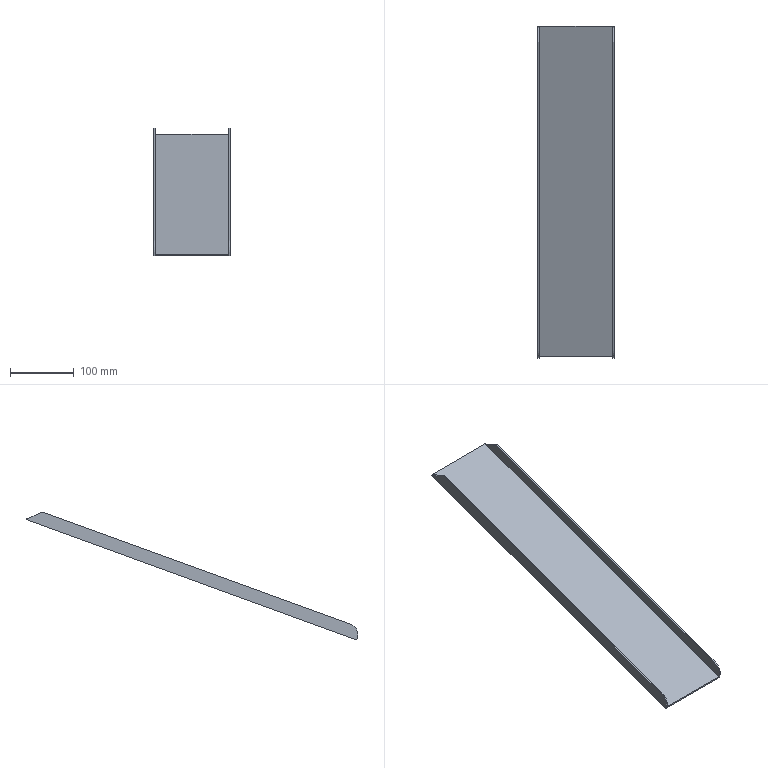Part | NX | features solid 2 | 1 solid | 16 faces | box 120 x 521.77 x 201.218 mm | volume 171498 mm3 | plane 14 | cylinder 2 | commonest cylinder face diameters 36 x2
STEP:
#1=CARTESIAN_POINT('',(782.,-610.,-362.136));
#2=VERTEX_POINT('',#1);
#3=CARTESIAN_POINT('',(898.,-610.,-362.136));
#4=VERTEX_POINT('',#3);
#5=CARTESIAN_POINT('',(770.,-610.,-362.136));
#6=DIRECTION('',(-1.,0.,0.));
#7=VECTOR('',#6,1000.);
#8=LINE('',#5,#7);
#9=EDGE_CURVE('',#2,#4,#8,.F.);
#10=ORIENTED_EDGE('',*,*,#9,.F.);
#11=CARTESIAN_POINT('',(782.,-610.,-364.265));
#12=VERTEX_POINT('',#11);
#13=CARTESIAN_POINT('',(782.,-610.,-155.));
#14=DIRECTION('',(0.,0.,1.));
#15=VECTOR('',#14,1000.);
#16=LINE('',#13,#15);
#17=EDGE_CURVE('',#2,#12,#16,.F.);
#18=ORIENTED_EDGE('',*,*,#17,.T.);
#19=CARTESIAN_POINT('',(898.,-610.,-364.265));
#20=VERTEX_POINT('',#19);
#21=CARTESIAN_POINT('',(770.,-610.,-364.265));
#22=DIRECTION('',(-1.,0.,0.));
#23=VECTOR('',#22,1000.);
#24=LINE('',#21,#23);
#25=EDGE_CURVE('',#12,#20,#24,.F.);
#26=ORIENTED_EDGE('',*,*,#25,.T.);
#27=CARTESIAN_POINT('',(898.,-610.,-155.));
#28=DIRECTION('',(0.,0.,1.));
#29=VECTOR('',#28,1000.);
#30=LINE('',#27,#29);
#31=EDGE_CURVE('',#4,#20,#30,.F.);
#32=ORIENTED_EDGE('',*,*,#31,.F.);
#33=EDGE_LOOP('',(#10,#18,#26,#32));
#34=FACE_BOUND('',#33,.T.);
#35=CARTESIAN_POINT('',(1030.,-610.,-155.));
#36=DIRECTION('',(0.,-1.,0.));
#37=DIRECTION('',(0.,0.,-1.));
#38=AXIS2_PLACEMENT_3D('',#35,#36,#37);
#39=PLANE('',#38);
#40=ADVANCED_FACE('',(#34),#39,.T.);
#41=CARTESIAN_POINT('',(898.,-92.563,-173.805));
#42=VERTEX_POINT('',#41);
#43=CARTESIAN_POINT('',(898.,-323.643,-257.911));
#44=DIRECTION('',(0.,0.9397,0.342));
#45=VECTOR('',#44,1000.);
#46=LINE('',#43,#45);
#47=EDGE_CURVE('',#4,#42,#46,.T.);
#48=ORIENTED_EDGE('',*,*,#47,.T.);
#49=CARTESIAN_POINT('',(900.,-92.563,-173.805));
#50=VERTEX_POINT('',#49);
#51=CARTESIAN_POINT('',(770.,-92.563,-173.805));
#52=DIRECTION('',(1.,0.,0.));
#53=VECTOR('',#52,1000.);
#54=LINE('',#51,#53);
#55=EDGE_CURVE('',#42,#50,#54,.T.);
#56=ORIENTED_EDGE('',*,*,#55,.T.);
#57=CARTESIAN_POINT('',(900.,-90.684,-173.121));
#58=VERTEX_POINT('',#57);
#59=CARTESIAN_POINT('',(900.,-323.643,-257.911));
#60=DIRECTION('',(0.,0.9397,0.342));
#61=VECTOR('',#60,1000.);
#62=LINE('',#59,#61);
#63=EDGE_CURVE('',#50,#58,#62,.T.);
#64=ORIENTED_EDGE('',*,*,#63,.T.);
#65=CARTESIAN_POINT('',(780.,-90.684,-173.121));
#66=VERTEX_POINT('',#65);
#67=CARTESIAN_POINT('',(770.,-90.684,-173.121));
#68=DIRECTION('',(-1.,0.,0.));
#69=VECTOR('',#68,1000.);
#70=LINE('',#67,#69);
#71=EDGE_CURVE('',#66,#58,#70,.F.);
#72=ORIENTED_EDGE('',*,*,#71,.F.);
#73=CARTESIAN_POINT('',(780.,-92.563,-173.805));
#74=VERTEX_POINT('',#73);
#75=CARTESIAN_POINT('',(780.,-323.643,-257.911));
#76=DIRECTION('',(0.,0.9397,0.342));
#77=VECTOR('',#76,1000.);
#78=LINE('',#75,#77);
#79=EDGE_CURVE('',#74,#66,#78,.T.);
#80=ORIENTED_EDGE('',*,*,#79,.F.);
#81=CARTESIAN_POINT('',(782.,-92.563,-173.805));
#82=VERTEX_POINT('',#81);
#83=CARTESIAN_POINT('',(770.,-92.563,-173.805));
#84=DIRECTION('',(1.,0.,0.));
#85=VECTOR('',#84,1000.);
#86=LINE('',#83,#85);
#87=EDGE_CURVE('',#74,#82,#86,.T.);
#88=ORIENTED_EDGE('',*,*,#87,.T.);
#89=CARTESIAN_POINT('',(782.,-323.643,-257.911));
#90=DIRECTION('',(0.,0.9397,0.342));
#91=VECTOR('',#90,1000.);
#92=LINE('',#89,#91);
#93=EDGE_CURVE('',#2,#82,#92,.T.);
#94=ORIENTED_EDGE('',*,*,#93,.F.);
#95=ORIENTED_EDGE('',*,*,#9,.T.);
#96=EDGE_LOOP('',(#48,#56,#64,#72,#80,#88,#94,#95));
#97=FACE_BOUND('',#96,.T.);
#98=CARTESIAN_POINT('',(770.,-323.643,-257.911));
#99=DIRECTION('',(0.,-0.342,0.9397));
#100=DIRECTION('',(0.,0.9397,0.342));
#101=AXIS2_PLACEMENT_3D('',#98,#99,#100);
#102=PLANE('',#101);
#103=ADVANCED_FACE('',(#97),#102,.T.);
#104=ORIENTED_EDGE('',*,*,#71,.T.);
#105=CARTESIAN_POINT('',(900.,-90.,-175.));
#106=VERTEX_POINT('',#105);
#107=CARTESIAN_POINT('',(900.,-110.521,-118.618));
#108=DIRECTION('',(0.,-0.342,0.9397));
#109=VECTOR('',#108,1000.);
#110=LINE('',#107,#109);
#111=EDGE_CURVE('',#58,#106,#110,.F.);
#112=ORIENTED_EDGE('',*,*,#111,.T.);
#113=CARTESIAN_POINT('',(780.,-90.,-175.));
#114=VERTEX_POINT('',#113);
#115=CARTESIAN_POINT('',(770.,-90.,-175.));
#116=DIRECTION('',(-1.,0.,0.));
#117=VECTOR('',#116,1000.);
#118=LINE('',#115,#117);
#119=EDGE_CURVE('',#114,#106,#118,.F.);
#120=ORIENTED_EDGE('',*,*,#119,.F.);
#121=CARTESIAN_POINT('',(780.,-110.521,-118.618));
#122=DIRECTION('',(0.,-0.342,0.9397));
#123=VECTOR('',#122,1000.);
#124=LINE('',#121,#123);
#125=EDGE_CURVE('',#66,#114,#124,.F.);
#126=ORIENTED_EDGE('',*,*,#125,.F.);
#127=EDGE_LOOP('',(#104,#112,#120,#126));
#128=FACE_BOUND('',#127,.T.);
#129=CARTESIAN_POINT('',(770.,-110.521,-118.618));
#130=DIRECTION('',(0.,0.9397,0.342));
#131=DIRECTION('',(0.,0.342,-0.9397));
#132=AXIS2_PLACEMENT_3D('',#129,#130,#131);
#133=PLANE('',#132);
#134=ADVANCED_FACE('',(#128),#133,.T.);
#135=ORIENTED_EDGE('',*,*,#25,.F.);
#136=CARTESIAN_POINT('',(780.,-610.,-364.265));
#137=VERTEX_POINT('',#136);
#138=CARTESIAN_POINT('',(770.,-610.,-364.265));
#139=DIRECTION('',(-1.,0.,0.));
#140=VECTOR('',#139,1000.);
#141=LINE('',#138,#140);
#142=EDGE_CURVE('',#137,#12,#141,.F.);
#143=ORIENTED_EDGE('',*,*,#142,.F.);
#144=CARTESIAN_POINT('',(780.,-322.959,-259.79));
#145=DIRECTION('',(0.,0.9397,0.342));
#146=VECTOR('',#145,1000.);
#147=LINE('',#144,#146);
#148=EDGE_CURVE('',#137,#114,#147,.T.);
#149=ORIENTED_EDGE('',*,*,#148,.T.);
#150=ORIENTED_EDGE('',*,*,#119,.T.);
#151=CARTESIAN_POINT('',(900.,-610.,-364.265));
#152=VERTEX_POINT('',#151);
#153=CARTESIAN_POINT('',(900.,-322.959,-259.79));
#154=DIRECTION('',(0.,0.9397,0.342));
#155=VECTOR('',#154,1000.);
#156=LINE('',#153,#155);
#157=EDGE_CURVE('',#152,#106,#156,.T.);
#158=ORIENTED_EDGE('',*,*,#157,.F.);
#159=CARTESIAN_POINT('',(900.,-610.,-364.265));
#160=DIRECTION('',(-1.,0.,0.));
#161=VECTOR('',#160,1000.);
#162=LINE('',#159,#161);
#163=EDGE_CURVE('',#152,#20,#162,.T.);
#164=ORIENTED_EDGE('',*,*,#163,.T.);
#165=EDGE_LOOP('',(#135,#143,#149,#150,#158,#164));
#166=FACE_BOUND('',#165,.T.);
#167=CARTESIAN_POINT('',(770.,-322.959,-259.79));
#168=DIRECTION('',(0.,-0.342,0.9397));
#169=DIRECTION('',(0.,0.9397,0.342));
#170=AXIS2_PLACEMENT_3D('',#167,#168,#169);
#171=PLANE('',#170);
#172=ADVANCED_FACE('',(#166),#171,.F.);
#173=ORIENTED_EDGE('',*,*,#157,.T.);
#174=ORIENTED_EDGE('',*,*,#111,.F.);
#175=ORIENTED_EDGE('',*,*,#63,.F.);
#176=CARTESIAN_POINT('',(900.,-115.634,-163.047));
#177=VERTEX_POINT('',#176);
#178=CARTESIAN_POINT('',(900.,-90.,-175.));
#179=DIRECTION('',(0.,0.9063,-0.4226));
#180=VECTOR('',#179,1000.);
#181=LINE('',#178,#180);
#182=EDGE_CURVE('',#177,#50,#181,.T.);
#183=ORIENTED_EDGE('',*,*,#182,.F.);
#184=CARTESIAN_POINT('',(900.,-599.926,-339.314));
#185=VERTEX_POINT('',#184);
#186=CARTESIAN_POINT('',(900.,-616.84,-345.471));
#187=DIRECTION('',(0.,0.9397,0.342));
#188=VECTOR('',#187,1000.);
#189=LINE('',#186,#188);
#190=EDGE_CURVE('',#185,#177,#189,.T.);
#191=ORIENTED_EDGE('',*,*,#190,.F.);
#192=CARTESIAN_POINT('',(900.,-610.684,-362.385));
#193=VERTEX_POINT('',#192);
#194=CARTESIAN_POINT('',(900.,-593.77,-356.229));
#195=DIRECTION('',(1.,0.,0.));
#196=DIRECTION('',(0.,0.,-1.));
#197=AXIS2_PLACEMENT_3D('',#194,#195,#196);
#198=CIRCLE('',#197,18.);
#199=EDGE_CURVE('',#193,#185,#198,.F.);
#200=ORIENTED_EDGE('',*,*,#199,.F.);
#201=CARTESIAN_POINT('',(900.,-610.,-364.265));
#202=DIRECTION('',(0.,-0.342,0.9397));
#203=VECTOR('',#202,1000.);
#204=LINE('',#201,#203);
#205=EDGE_CURVE('',#152,#193,#204,.T.);
#206=ORIENTED_EDGE('',*,*,#205,.F.);
#207=EDGE_LOOP('',(#173,#174,#175,#183,#191,#200,#206));
#208=FACE_BOUND('',#207,.T.);
#209=CARTESIAN_POINT('',(900.,-343.481,-203.409));
#210=DIRECTION('',(-1.,0.,0.));
#211=DIRECTION('',(0.,-0.342,0.9397));
#212=AXIS2_PLACEMENT_3D('',#209,#210,#211);
#213=PLANE('',#212);
#214=ADVANCED_FACE('',(#208),#213,.F.);
#215=CARTESIAN_POINT('',(780.,-610.684,-362.385));
#216=VERTEX_POINT('',#215);
#217=CARTESIAN_POINT('',(780.,-610.,-364.265));
#218=DIRECTION('',(0.,-0.342,0.9397));
#219=VECTOR('',#218,1000.);
#220=LINE('',#217,#219);
#221=EDGE_CURVE('',#137,#216,#220,.T.);
#222=ORIENTED_EDGE('',*,*,#221,.T.);
#223=CARTESIAN_POINT('',(780.,-599.926,-339.314));
#224=VERTEX_POINT('',#223);
#225=CARTESIAN_POINT('',(780.,-593.77,-356.229));
#226=DIRECTION('',(1.,0.,0.));
#227=DIRECTION('',(0.,0.,-1.));
#228=AXIS2_PLACEMENT_3D('',#225,#226,#227);
#229=CIRCLE('',#228,18.);
#230=EDGE_CURVE('',#224,#216,#229,.T.);
#231=ORIENTED_EDGE('',*,*,#230,.F.);
#232=CARTESIAN_POINT('',(780.,-115.634,-163.047));
#233=VERTEX_POINT('',#232);
#234=CARTESIAN_POINT('',(780.,-616.84,-345.471));
#235=DIRECTION('',(0.,0.9397,0.342));
#236=VECTOR('',#235,1000.);
#237=LINE('',#234,#236);
#238=EDGE_CURVE('',#224,#233,#237,.T.);
#239=ORIENTED_EDGE('',*,*,#238,.T.);
#240=CARTESIAN_POINT('',(780.,-444.632,-9.632));
#241=DIRECTION('',(0.,-0.9063,0.4226));
#242=VECTOR('',#241,1000.);
#243=LINE('',#240,#242);
#244=EDGE_CURVE('',#74,#233,#243,.T.);
#245=ORIENTED_EDGE('',*,*,#244,.F.);
#246=ORIENTED_EDGE('',*,*,#79,.T.);
#247=ORIENTED_EDGE('',*,*,#125,.T.);
#248=ORIENTED_EDGE('',*,*,#148,.F.);
#249=EDGE_LOOP('',(#222,#231,#239,#245,#246,#247,#248));
#250=FACE_BOUND('',#249,.T.);
#251=CARTESIAN_POINT('',(780.,-343.481,-203.409));
#252=DIRECTION('',(-1.,0.,0.));
#253=DIRECTION('',(0.,-0.342,0.9397));
#254=AXIS2_PLACEMENT_3D('',#251,#252,#253);
#255=PLANE('',#254);
#256=ADVANCED_FACE('',(#250),#255,.T.);
#257=ORIENTED_EDGE('',*,*,#93,.T.);
#258=CARTESIAN_POINT('',(782.,-115.634,-163.047));
#259=VERTEX_POINT('',#258);
#260=CARTESIAN_POINT('',(782.,-115.634,-163.047));
#261=DIRECTION('',(0.,0.9063,-0.4226));
#262=VECTOR('',#261,1000.);
#263=LINE('',#260,#262);
#264=EDGE_CURVE('',#259,#82,#263,.T.);
#265=ORIENTED_EDGE('',*,*,#264,.F.);
#266=CARTESIAN_POINT('',(782.,-599.926,-339.314));
#267=VERTEX_POINT('',#266);
#268=CARTESIAN_POINT('',(782.,-616.84,-345.471));
#269=DIRECTION('',(0.,0.9397,0.342));
#270=VECTOR('',#269,1000.);
#271=LINE('',#268,#270);
#272=EDGE_CURVE('',#267,#259,#271,.T.);
#273=ORIENTED_EDGE('',*,*,#272,.F.);
#274=CARTESIAN_POINT('',(782.,-610.684,-362.385));
#275=VERTEX_POINT('',#274);
#276=CARTESIAN_POINT('',(782.,-593.77,-356.229));
#277=DIRECTION('',(1.,0.,0.));
#278=DIRECTION('',(0.,0.,-1.));
#279=AXIS2_PLACEMENT_3D('',#276,#277,#278);
#280=CIRCLE('',#279,18.);
#281=EDGE_CURVE('',#275,#267,#280,.F.);
#282=ORIENTED_EDGE('',*,*,#281,.F.);
#283=CARTESIAN_POINT('',(782.,-610.,-364.265));
#284=DIRECTION('',(0.,-0.342,0.9397));
#285=VECTOR('',#284,1000.);
#286=LINE('',#283,#285);
#287=EDGE_CURVE('',#12,#275,#286,.T.);
#288=ORIENTED_EDGE('',*,*,#287,.F.);
#289=ORIENTED_EDGE('',*,*,#17,.F.);
#290=EDGE_LOOP('',(#257,#265,#273,#282,#288,#289));
#291=FACE_BOUND('',#290,.T.);
#292=CARTESIAN_POINT('',(782.,-610.,-364.265));
#293=DIRECTION('',(-1.,0.,0.));
#294=DIRECTION('',(0.,0.,-1.));
#295=AXIS2_PLACEMENT_3D('',#292,#293,#294);
#296=PLANE('',#295);
#297=ADVANCED_FACE('',(#291),#296,.F.);
#298=ORIENTED_EDGE('',*,*,#238,.F.);
#299=CARTESIAN_POINT('',(780.,-599.926,-339.314));
#300=DIRECTION('',(1.,0.,0.));
#301=VECTOR('',#300,1000.);
#302=LINE('',#299,#301);
#303=EDGE_CURVE('',#267,#224,#302,.F.);
#304=ORIENTED_EDGE('',*,*,#303,.F.);
#305=ORIENTED_EDGE('',*,*,#272,.T.);
#306=CARTESIAN_POINT('',(780.,-115.634,-163.047));
#307=DIRECTION('',(1.,0.,0.));
#308=VECTOR('',#307,1000.);
#309=LINE('',#306,#308);
#310=EDGE_CURVE('',#233,#259,#309,.T.);
#311=ORIENTED_EDGE('',*,*,#310,.F.);
#312=EDGE_LOOP('',(#298,#304,#305,#311));
#313=FACE_BOUND('',#312,.T.);
#314=CARTESIAN_POINT('',(780.,-616.84,-345.471));
#315=DIRECTION('',(0.,0.342,-0.9397));
#316=DIRECTION('',(0.,0.9397,0.342));
#317=AXIS2_PLACEMENT_3D('',#314,#315,#316);
#318=PLANE('',#317);
#319=ADVANCED_FACE('',(#313),#318,.F.);
#320=ORIENTED_EDGE('',*,*,#221,.F.);
#321=ORIENTED_EDGE('',*,*,#142,.T.);
#322=ORIENTED_EDGE('',*,*,#287,.T.);
#323=CARTESIAN_POINT('',(780.,-610.684,-362.385));
#324=DIRECTION('',(1.,0.,0.));
#325=VECTOR('',#324,1000.);
#326=LINE('',#323,#325);
#327=EDGE_CURVE('',#216,#275,#326,.T.);
#328=ORIENTED_EDGE('',*,*,#327,.F.);
#329=EDGE_LOOP('',(#320,#321,#322,#328));
#330=FACE_BOUND('',#329,.T.);
#331=CARTESIAN_POINT('',(780.,-610.,-364.265));
#332=DIRECTION('',(0.,0.9397,0.342));
#333=DIRECTION('',(0.,-0.342,0.9397));
#334=AXIS2_PLACEMENT_3D('',#331,#332,#333);
#335=PLANE('',#334);
#336=ADVANCED_FACE('',(#330),#335,.F.);
#337=ORIENTED_EDGE('',*,*,#230,.T.);
#338=ORIENTED_EDGE('',*,*,#327,.T.);
#339=ORIENTED_EDGE('',*,*,#281,.T.);
#340=ORIENTED_EDGE('',*,*,#303,.T.);
#341=EDGE_LOOP('',(#337,#338,#339,#340));
#342=FACE_BOUND('',#341,.T.);
#343=CARTESIAN_POINT('',(780.,-593.77,-356.229));
#344=DIRECTION('',(1.,0.,0.));
#345=DIRECTION('',(0.,0.,1.));
#346=AXIS2_PLACEMENT_3D('',#343,#344,#345);
#347=CYLINDRICAL_SURFACE('',#346,18.);
#348=ADVANCED_FACE('',(#342),#347,.T.);
#349=ORIENTED_EDGE('',*,*,#244,.T.);
#350=ORIENTED_EDGE('',*,*,#310,.T.);
#351=ORIENTED_EDGE('',*,*,#264,.T.);
#352=ORIENTED_EDGE('',*,*,#87,.F.);
#353=EDGE_LOOP('',(#349,#350,#351,#352));
#354=FACE_BOUND('',#353,.T.);
#355=CARTESIAN_POINT('',(780.,-115.634,-163.047));
#356=DIRECTION('',(0.,0.4226,0.9063));
#357=DIRECTION('',(0.,-0.9063,0.4226));
#358=AXIS2_PLACEMENT_3D('',#355,#356,#357);
#359=PLANE('',#358);
#360=ADVANCED_FACE('',(#354),#359,.T.);
#361=ORIENTED_EDGE('',*,*,#31,.T.);
#362=CARTESIAN_POINT('',(898.,-610.684,-362.385));
#363=VERTEX_POINT('',#362);
#364=CARTESIAN_POINT('',(898.,-610.,-364.265));
#365=DIRECTION('',(0.,-0.342,0.9397));
#366=VECTOR('',#365,1000.);
#367=LINE('',#364,#366);
#368=EDGE_CURVE('',#20,#363,#367,.T.);
#369=ORIENTED_EDGE('',*,*,#368,.T.);
#370=CARTESIAN_POINT('',(898.,-599.926,-339.314));
#371=VERTEX_POINT('',#370);
#372=CARTESIAN_POINT('',(898.,-593.77,-356.229));
#373=DIRECTION('',(1.,0.,0.));
#374=DIRECTION('',(0.,0.,-1.));
#375=AXIS2_PLACEMENT_3D('',#372,#373,#374);
#376=CIRCLE('',#375,18.);
#377=EDGE_CURVE('',#371,#363,#376,.T.);
#378=ORIENTED_EDGE('',*,*,#377,.F.);
#379=CARTESIAN_POINT('',(898.,-115.634,-163.047));
#380=VERTEX_POINT('',#379);
#381=CARTESIAN_POINT('',(898.,-616.84,-345.471));
#382=DIRECTION('',(0.,0.9397,0.342));
#383=VECTOR('',#382,1000.);
#384=LINE('',#381,#383);
#385=EDGE_CURVE('',#371,#380,#384,.T.);
#386=ORIENTED_EDGE('',*,*,#385,.T.);
#387=CARTESIAN_POINT('',(898.,-444.632,-9.632));
#388=DIRECTION('',(0.,-0.9063,0.4226));
#389=VECTOR('',#388,1000.);
#390=LINE('',#387,#389);
#391=EDGE_CURVE('',#42,#380,#390,.T.);
#392=ORIENTED_EDGE('',*,*,#391,.F.);
#393=ORIENTED_EDGE('',*,*,#47,.F.);
#394=EDGE_LOOP('',(#361,#369,#378,#386,#392,#393));
#395=FACE_BOUND('',#394,.T.);
#396=CARTESIAN_POINT('',(898.,-610.,-364.265));
#397=DIRECTION('',(-1.,0.,0.));
#398=DIRECTION('',(0.,0.,-1.));
#399=AXIS2_PLACEMENT_3D('',#396,#397,#398);
#400=PLANE('',#399);
#401=ADVANCED_FACE('',(#395),#400,.T.);
#402=ORIENTED_EDGE('',*,*,#385,.F.);
#403=CARTESIAN_POINT('',(900.,-599.926,-339.314));
#404=DIRECTION('',(1.,0.,0.));
#405=VECTOR('',#404,1000.);
#406=LINE('',#403,#405);
#407=EDGE_CURVE('',#185,#371,#406,.F.);
#408=ORIENTED_EDGE('',*,*,#407,.F.);
#409=ORIENTED_EDGE('',*,*,#190,.T.);
#410=CARTESIAN_POINT('',(900.,-115.634,-163.047));
#411=DIRECTION('',(-1.,0.,0.));
#412=VECTOR('',#411,1000.);
#413=LINE('',#410,#412);
#414=EDGE_CURVE('',#380,#177,#413,.F.);
#415=ORIENTED_EDGE('',*,*,#414,.F.);
#416=EDGE_LOOP('',(#402,#408,#409,#415));
#417=FACE_BOUND('',#416,.T.);
#418=CARTESIAN_POINT('',(900.,-616.84,-345.471));
#419=DIRECTION('',(0.,0.342,-0.9397));
#420=DIRECTION('',(0.,0.9397,0.342));
#421=AXIS2_PLACEMENT_3D('',#418,#419,#420);
#422=PLANE('',#421);
#423=ADVANCED_FACE('',(#417),#422,.F.);
#424=ORIENTED_EDGE('',*,*,#368,.F.);
#425=ORIENTED_EDGE('',*,*,#163,.F.);
#426=ORIENTED_EDGE('',*,*,#205,.T.);
#427=CARTESIAN_POINT('',(900.,-610.684,-362.385));
#428=DIRECTION('',(1.,0.,0.));
#429=VECTOR('',#428,1000.);
#430=LINE('',#427,#429);
#431=EDGE_CURVE('',#363,#193,#430,.T.);
#432=ORIENTED_EDGE('',*,*,#431,.F.);
#433=EDGE_LOOP('',(#424,#425,#426,#432));
#434=FACE_BOUND('',#433,.T.);
#435=CARTESIAN_POINT('',(900.,-610.,-364.265));
#436=DIRECTION('',(0.,0.9397,0.342));
#437=DIRECTION('',(0.,-0.342,0.9397));
#438=AXIS2_PLACEMENT_3D('',#435,#436,#437);
#439=PLANE('',#438);
#440=ADVANCED_FACE('',(#434),#439,.F.);
#441=ORIENTED_EDGE('',*,*,#199,.T.);
#442=ORIENTED_EDGE('',*,*,#407,.T.);
#443=ORIENTED_EDGE('',*,*,#377,.T.);
#444=ORIENTED_EDGE('',*,*,#431,.T.);
#445=EDGE_LOOP('',(#441,#442,#443,#444));
#446=FACE_BOUND('',#445,.T.);
#447=CARTESIAN_POINT('',(900.,-593.77,-356.229));
#448=DIRECTION('',(-1.,0.,0.));
#449=DIRECTION('',(0.,0.,-1.));
#450=AXIS2_PLACEMENT_3D('',#447,#448,#449);
#451=CYLINDRICAL_SURFACE('',#450,18.);
#452=ADVANCED_FACE('',(#446),#451,.T.);
#453=ORIENTED_EDGE('',*,*,#391,.T.);
#454=ORIENTED_EDGE('',*,*,#414,.T.);
#455=ORIENTED_EDGE('',*,*,#182,.T.);
#456=ORIENTED_EDGE('',*,*,#55,.F.);
#457=EDGE_LOOP('',(#453,#454,#455,#456));
#458=FACE_BOUND('',#457,.T.);
#459=CARTESIAN_POINT('',(900.,-90.,-175.));
#460=DIRECTION('',(0.,0.4226,0.9063));
#461=DIRECTION('',(0.,-0.9063,0.4226));
#462=AXIS2_PLACEMENT_3D('',#459,#460,#461);
#463=PLANE('',#462);
#464=ADVANCED_FACE('',(#458),#463,.T.);
#465=CLOSED_SHELL('',(#40,#103,#134,#172,#214,#256,#297,#319,#336,#348,#360,#401,#423,#440,#452,#464));
#466=MANIFOLD_SOLID_BREP('',#465);
#467=(LENGTH_UNIT()NAMED_UNIT(*)SI_UNIT(.MILLI.,.METRE.));
#468=UNCERTAINTY_MEASURE_WITH_UNIT(LENGTH_MEASURE(0.00001),#467,'','');
#469=(NAMED_UNIT(*)PLANE_ANGLE_UNIT()SI_UNIT($,.RADIAN.));
#470=(NAMED_UNIT(*)SI_UNIT($,.STERADIAN.)SOLID_ANGLE_UNIT());
#471=(GEOMETRIC_REPRESENTATION_CONTEXT(3)GLOBAL_UNCERTAINTY_ASSIGNED_CONTEXT((#468))GLOBAL_UNIT_ASSIGNED_CONTEXT((#467,#469,#470))REPRESENTATION_CONTEXT('',''));
#472=ADVANCED_BREP_SHAPE_REPRESENTATION('',(#466),#471);